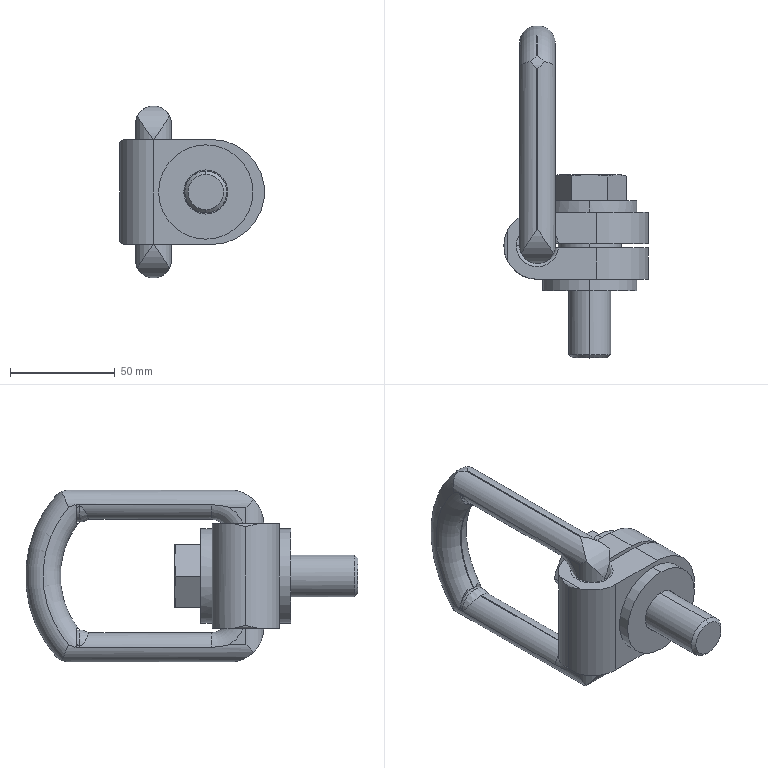Part | CATIA | 2 solids | 128 faces | box 69 x 158.5 x 82 mm | volume 178228 mm3 | plane 54 | cylinder 50 | torus 12 | cone 8 | sphere 4 | commonest cylinder face diameters 16.6 x14 30.1 x4 32 x4 45 x4 78 x4 3.2 x2